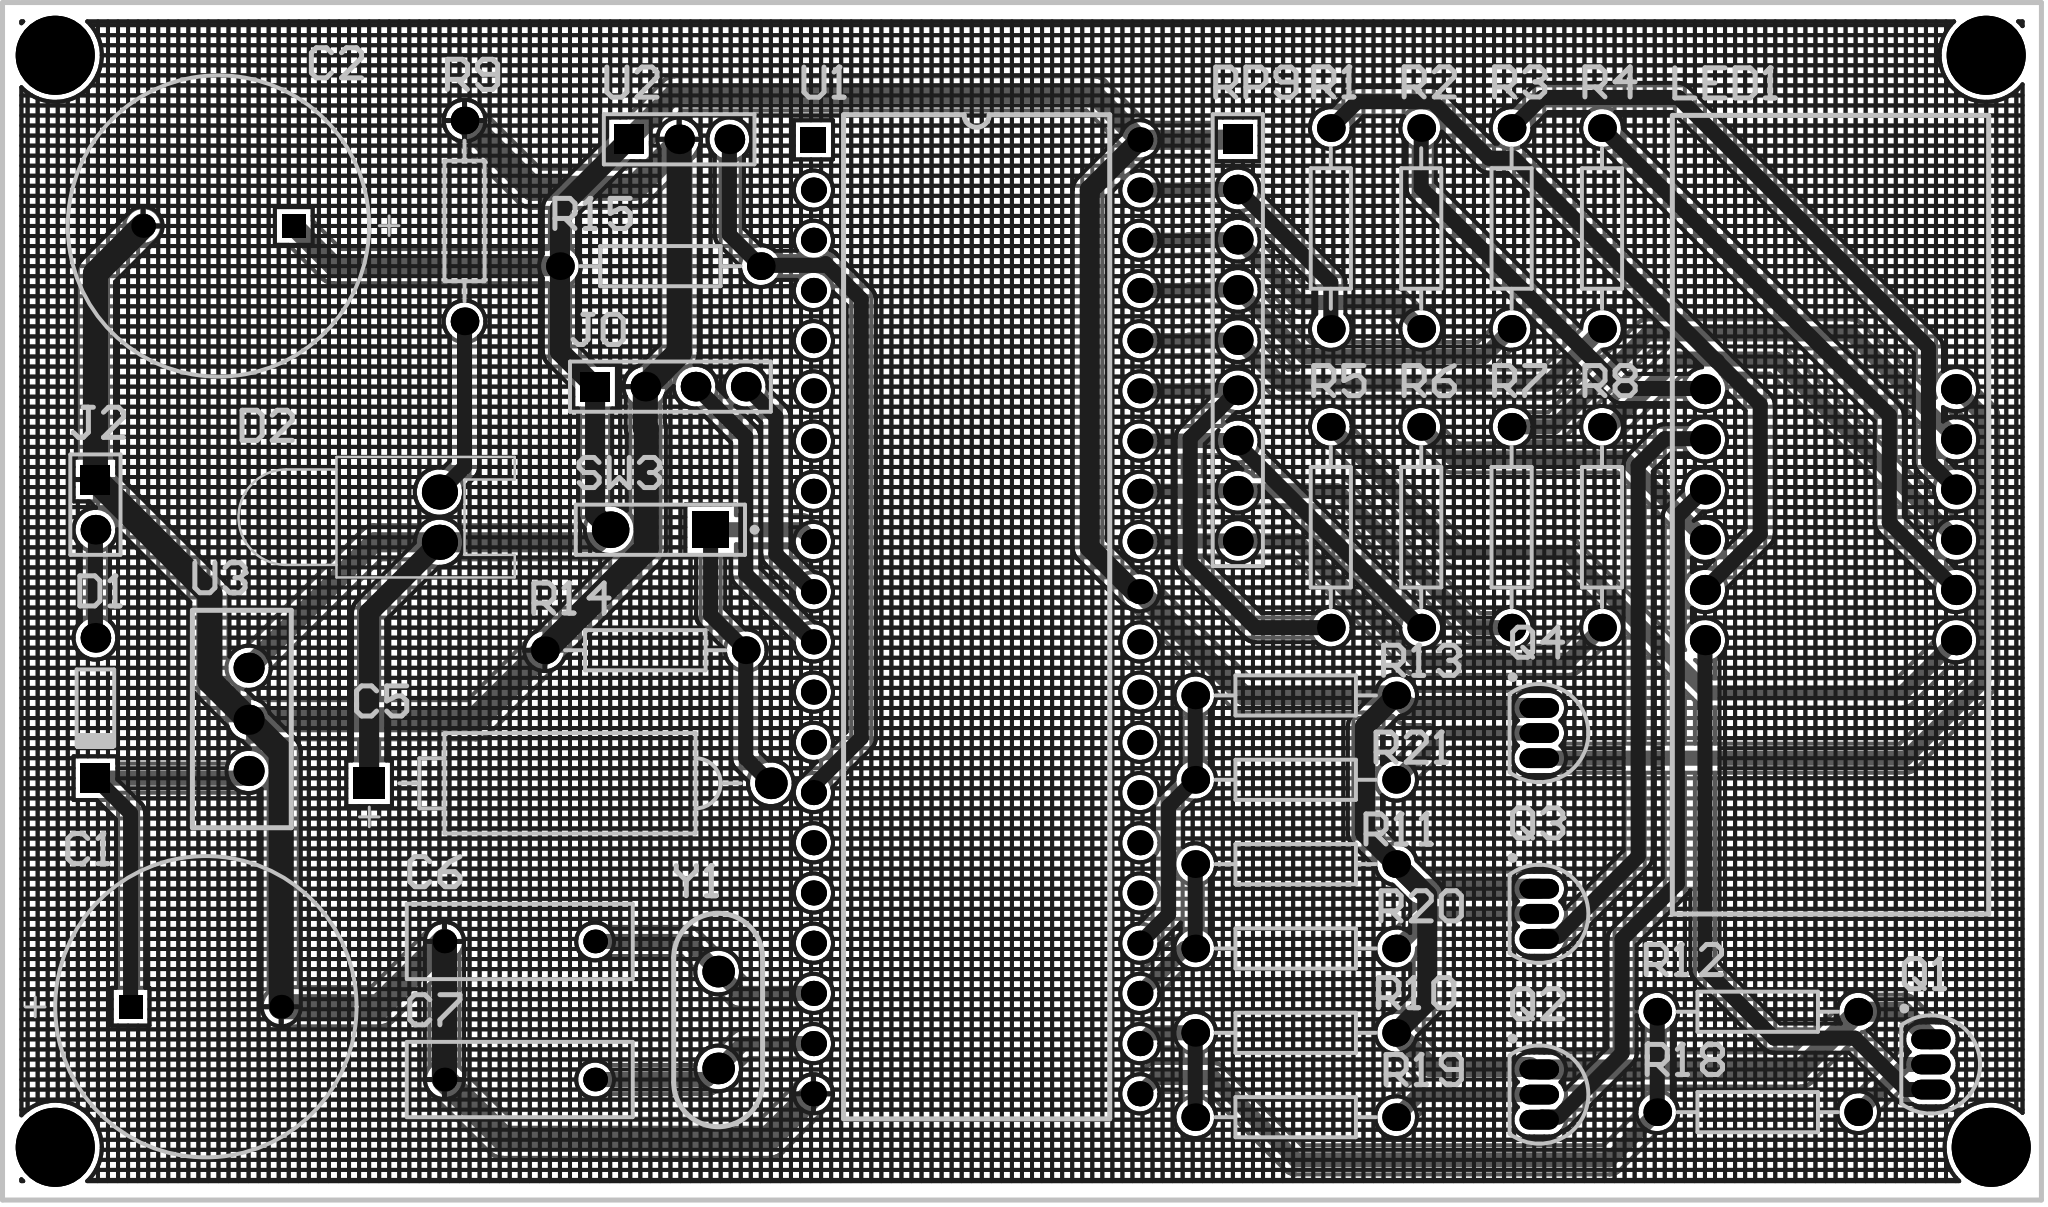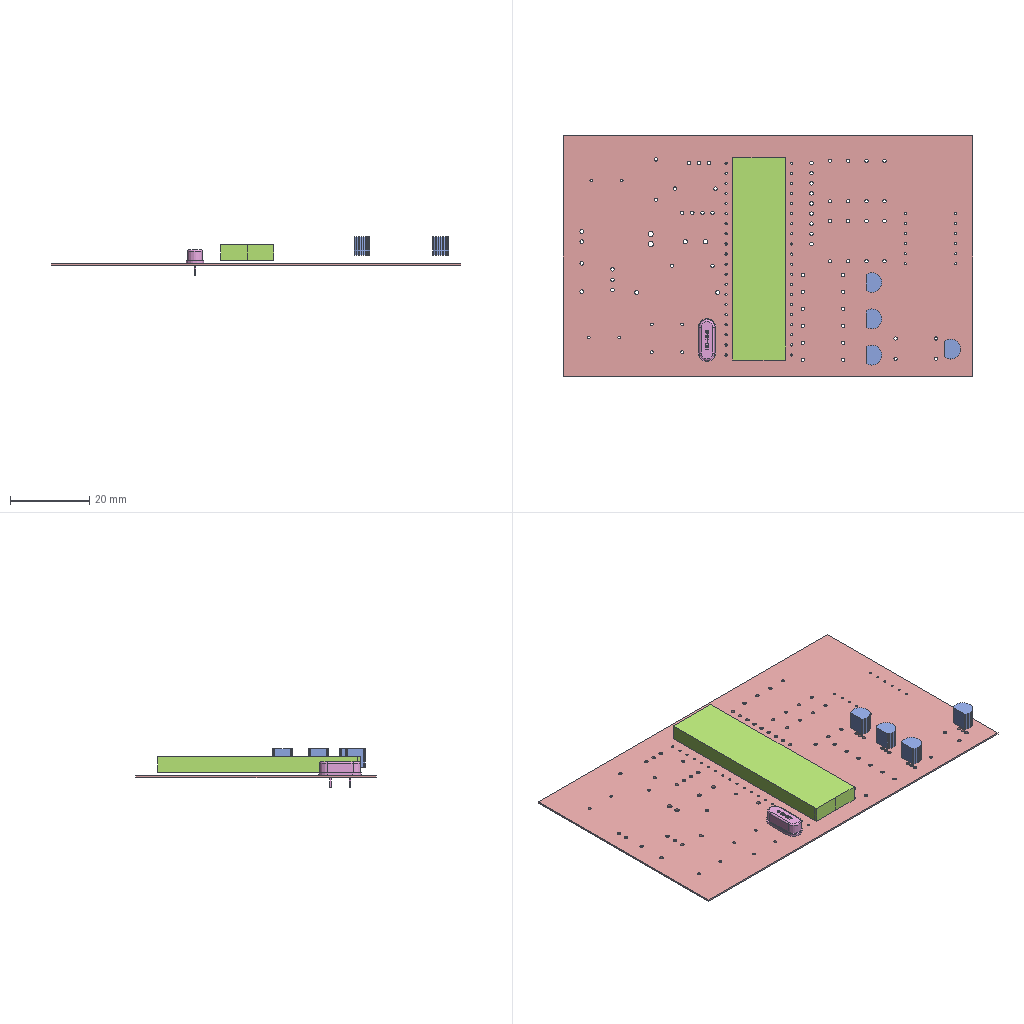Circuit board layout | Altium Designer | box 103.1 x 60.6 x 9.8 mm
Part placement:
Designator,Comment,Layer,Footprint,Center-X(mm),Center-Y(mm),Rotation
J0,Header 4,TopLayer,HDR1X4,81.788,99.568,360
C1,Cap Pol1,TopLayer,RB7.6-15,58.293,68.199,180
C2,Cap Pol1,TopLayer,RB7.6-15,58.928,107.696,360
C5,Cap Pol2,TopLayer,POLAR0.8,76.708,79.502,180
C6,Cap,TopLayer,RAD-0.3,74.168,71.501,180
C7,Cap,TopLayer,RAD-0.3,74.168,64.516,180
D1,Diode 1N914,TopLayer,DO-35,52.705,83.312,270
D2,LED0,TopLayer,LED-0,70.104,92.964,270
J2,Header 2,TopLayer,HDR1X2,52.705,93.599,270
LED1,Dpy Red-CA,TopLayer,SIWEI,140.462,93.091,90
Q1,2N3906,TopLayer,TO-92A,145.542,65.278,180
Q2,2N3906,TopLayer,TO-92A,125.73,63.754,180
Q3,2N3906,TopLayer,TO-92A,125.73,72.898,180
Q4,2N3906,TopLayer,TO-92A,125.73,82.042,180
R1,Res2,TopLayer,AXIAL-0.4,115.189,107.569,90
R2,Res2,TopLayer,AXIAL-0.4,119.761,107.569,90
R3,Res2,TopLayer,AXIAL-0.4,124.333,107.569,90
R4,Res2,TopLayer,AXIAL-0.4,128.905,107.569,90
R5,Res2,TopLayer,AXIAL-0.4,115.189,92.456,90
R6,Res2,TopLayer,AXIAL-0.4,119.761,92.456,90
R7,Res2,TopLayer,AXIAL-0.4,124.333,92.456,90
R8,Res2,TopLayer,AXIAL-0.4,128.905,92.456,90
R9,Res2,TopLayer,AXIAL-0.4,71.374,107.95,90
R10,Res2,TopLayer,AXIAL-0.4,113.411,66.878,180
R11,Res2,TopLayer,AXIAL-0.4,113.411,75.413,180
R12,Res2,TopLayer,AXIAL-0.4,136.779,67.945,180
R13,Res2,TopLayer,AXIAL-0.4,113.411,83.947,180
R14,Res2,TopLayer,AXIAL-0.4,80.518,86.233,180
R15,Res2,TopLayer,AXIAL-0.4,81.28,105.664,180
R18,Res2,TopLayer,AXIAL-0.4,136.779,62.865,180
R19,Res2,TopLayer,AXIAL-0.4,113.411,62.611,180
R20,Res2,TopLayer,AXIAL-0.4,113.411,71.145,180
R21,Res2,TopLayer,AXIAL-0.4,113.411,79.68,180
RP9,20k,TopLayer,HDR1X9,110.484,101.921,270
SW3,SW-PB,TopLayer,SPST-2,81.28,92.329,180
U1,89c51,TopLayer,89c51,97.276,87.924,360
U2,AH49E,TopLayer,HDR1X3,82.23,112.081,360
U3,7805,TopLayer,PCBComponent_1,60.452,82.734,90
Y1,Component_1,TopLayer,LC-HC-49S,84.201,67.527,90